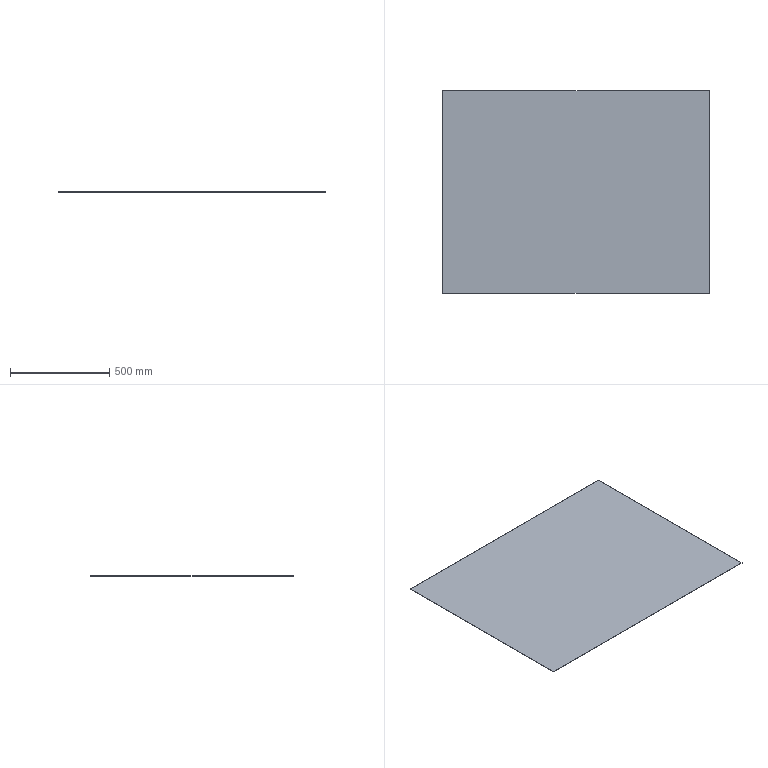Part | SolidWorks | features FlatPattern 1, SMBaseFlange 1, SheetMetal 1 | 1 solid | 6 faces | box 1345 x 1022 x 1.5 mm | volume 2062692 mm3 | plane 6
STEP:
#1=CARTESIAN_POINT('',(-672.5,0.,0.));
#2=VERTEX_POINT('',#1);
#3=CARTESIAN_POINT('',(-672.5,-1022.4,0.));
#4=VERTEX_POINT('',#3);
#5=CARTESIAN_POINT('',(-672.5,0.,0.));
#6=DIRECTION('',(0.,-1.,0.));
#7=VECTOR('',#6,1000.);
#8=LINE('',#5,#7);
#9=EDGE_CURVE('',#2,#4,#8,.T.);
#10=ORIENTED_EDGE('',*,*,#9,.T.);
#11=CARTESIAN_POINT('',(-672.5,-1022.4,1.5));
#12=VERTEX_POINT('',#11);
#13=CARTESIAN_POINT('',(-672.5,-1022.4,1.5));
#14=DIRECTION('',(0.,0.,-1.));
#15=VECTOR('',#14,1000.);
#16=LINE('',#13,#15);
#17=EDGE_CURVE('',#12,#4,#16,.T.);
#18=ORIENTED_EDGE('',*,*,#17,.F.);
#19=CARTESIAN_POINT('',(-672.5,0.,1.5));
#20=VERTEX_POINT('',#19);
#21=CARTESIAN_POINT('',(-672.5,0.,1.5));
#22=DIRECTION('',(0.,-1.,0.));
#23=VECTOR('',#22,1000.);
#24=LINE('',#21,#23);
#25=EDGE_CURVE('',#20,#12,#24,.T.);
#26=ORIENTED_EDGE('',*,*,#25,.F.);
#27=CARTESIAN_POINT('',(-672.5,0.,1.5));
#28=DIRECTION('',(0.,0.,-1.));
#29=VECTOR('',#28,1000.);
#30=LINE('',#27,#29);
#31=EDGE_CURVE('',#20,#2,#30,.T.);
#32=ORIENTED_EDGE('',*,*,#31,.T.);
#33=EDGE_LOOP('',(#10,#18,#26,#32));
#34=FACE_OUTER_BOUND('',#33,.T.);
#35=CARTESIAN_POINT('',(-672.5,0.,1.5));
#36=DIRECTION('',(1.,0.,0.));
#37=DIRECTION('',(0.,1.,0.));
#38=AXIS2_PLACEMENT_3D('',#35,#36,#37);
#39=PLANE('',#38);
#40=ADVANCED_FACE('',(#34),#39,.F.);
#41=CARTESIAN_POINT('',(672.5,-1022.4,0.));
#42=VERTEX_POINT('',#41);
#43=CARTESIAN_POINT('',(-672.5,-1022.4,0.));
#44=DIRECTION('',(1.,0.,0.));
#45=VECTOR('',#44,1000.);
#46=LINE('',#43,#45);
#47=EDGE_CURVE('',#4,#42,#46,.T.);
#48=ORIENTED_EDGE('',*,*,#47,.T.);
#49=CARTESIAN_POINT('',(672.5,-1022.4,1.5));
#50=VERTEX_POINT('',#49);
#51=CARTESIAN_POINT('',(672.5,-1022.4,1.5));
#52=DIRECTION('',(0.,0.,-1.));
#53=VECTOR('',#52,1000.);
#54=LINE('',#51,#53);
#55=EDGE_CURVE('',#50,#42,#54,.T.);
#56=ORIENTED_EDGE('',*,*,#55,.F.);
#57=CARTESIAN_POINT('',(-672.5,-1022.4,1.5));
#58=DIRECTION('',(1.,0.,0.));
#59=VECTOR('',#58,1000.);
#60=LINE('',#57,#59);
#61=EDGE_CURVE('',#12,#50,#60,.T.);
#62=ORIENTED_EDGE('',*,*,#61,.F.);
#63=ORIENTED_EDGE('',*,*,#17,.T.);
#64=EDGE_LOOP('',(#48,#56,#62,#63));
#65=FACE_OUTER_BOUND('',#64,.T.);
#66=CARTESIAN_POINT('',(-672.5,-1022.4,1.5));
#67=DIRECTION('',(0.,1.,0.));
#68=DIRECTION('',(0.,0.,1.));
#69=AXIS2_PLACEMENT_3D('',#66,#67,#68);
#70=PLANE('',#69);
#71=ADVANCED_FACE('',(#65),#70,.F.);
#72=CARTESIAN_POINT('',(672.5,0.,0.));
#73=VERTEX_POINT('',#72);
#74=CARTESIAN_POINT('',(672.5,0.,0.));
#75=DIRECTION('',(0.,1.,0.));
#76=VECTOR('',#75,1000.);
#77=LINE('',#74,#76);
#78=EDGE_CURVE('',#42,#73,#77,.T.);
#79=ORIENTED_EDGE('',*,*,#78,.T.);
#80=CARTESIAN_POINT('',(672.5,0.,1.5));
#81=VERTEX_POINT('',#80);
#82=CARTESIAN_POINT('',(672.5,0.,1.5));
#83=DIRECTION('',(0.,0.,-1.));
#84=VECTOR('',#83,1000.);
#85=LINE('',#82,#84);
#86=EDGE_CURVE('',#81,#73,#85,.T.);
#87=ORIENTED_EDGE('',*,*,#86,.F.);
#88=CARTESIAN_POINT('',(672.5,0.,1.5));
#89=DIRECTION('',(0.,1.,0.));
#90=VECTOR('',#89,1000.);
#91=LINE('',#88,#90);
#92=EDGE_CURVE('',#50,#81,#91,.T.);
#93=ORIENTED_EDGE('',*,*,#92,.F.);
#94=ORIENTED_EDGE('',*,*,#55,.T.);
#95=EDGE_LOOP('',(#79,#87,#93,#94));
#96=FACE_OUTER_BOUND('',#95,.T.);
#97=CARTESIAN_POINT('',(672.5,0.,1.5));
#98=DIRECTION('',(-1.,0.,0.));
#99=DIRECTION('',(0.,-1.,0.));
#100=AXIS2_PLACEMENT_3D('',#97,#98,#99);
#101=PLANE('',#100);
#102=ADVANCED_FACE('',(#96),#101,.F.);
#103=CARTESIAN_POINT('',(-672.5,0.,0.));
#104=DIRECTION('',(-1.,0.,0.));
#105=VECTOR('',#104,1000.);
#106=LINE('',#103,#105);
#107=EDGE_CURVE('',#73,#2,#106,.T.);
#108=ORIENTED_EDGE('',*,*,#107,.T.);
#109=ORIENTED_EDGE('',*,*,#31,.F.);
#110=CARTESIAN_POINT('',(-672.5,0.,1.5));
#111=DIRECTION('',(-1.,0.,0.));
#112=VECTOR('',#111,1000.);
#113=LINE('',#110,#112);
#114=EDGE_CURVE('',#81,#20,#113,.T.);
#115=ORIENTED_EDGE('',*,*,#114,.F.);
#116=ORIENTED_EDGE('',*,*,#86,.T.);
#117=EDGE_LOOP('',(#108,#109,#115,#116));
#118=FACE_OUTER_BOUND('',#117,.T.);
#119=CARTESIAN_POINT('',(-672.5,0.,1.5));
#120=DIRECTION('',(0.,-1.,0.));
#121=DIRECTION('',(1.,0.,0.));
#122=AXIS2_PLACEMENT_3D('',#119,#120,#121);
#123=PLANE('',#122);
#124=ADVANCED_FACE('',(#118),#123,.F.);
#125=ORIENTED_EDGE('',*,*,#25,.T.);
#126=ORIENTED_EDGE('',*,*,#61,.T.);
#127=ORIENTED_EDGE('',*,*,#92,.T.);
#128=ORIENTED_EDGE('',*,*,#114,.T.);
#129=EDGE_LOOP('',(#125,#126,#127,#128));
#130=FACE_OUTER_BOUND('',#129,.T.);
#131=CARTESIAN_POINT('',(0.,0.,1.5));
#132=DIRECTION('',(0.,0.,1.));
#133=DIRECTION('',(1.,0.,0.));
#134=AXIS2_PLACEMENT_3D('',#131,#132,#133);
#135=PLANE('',#134);
#136=ADVANCED_FACE('',(#130),#135,.T.);
#137=ORIENTED_EDGE('',*,*,#9,.F.);
#138=ORIENTED_EDGE('',*,*,#107,.F.);
#139=ORIENTED_EDGE('',*,*,#78,.F.);
#140=ORIENTED_EDGE('',*,*,#47,.F.);
#141=EDGE_LOOP('',(#137,#138,#139,#140));
#142=FACE_OUTER_BOUND('',#141,.T.);
#143=CARTESIAN_POINT('',(0.,0.,0.));
#144=DIRECTION('',(0.,0.,1.));
#145=DIRECTION('',(1.,0.,0.));
#146=AXIS2_PLACEMENT_3D('',#143,#144,#145);
#147=PLANE('',#146);
#148=ADVANCED_FACE('',(#142),#147,.F.);
#149=CLOSED_SHELL('',(#40,#71,#102,#124,#136,#148));
#150=MANIFOLD_SOLID_BREP('',#149);
#151=CARTESIAN_POINT('',(0.,0.,0.));
#152=DIRECTION('',(0.,0.,1.));
#153=DIRECTION('',(1.,0.,0.));
#154=AXIS2_PLACEMENT_3D('',#151,#152,#153);
#155=(LENGTH_UNIT()NAMED_UNIT(*)SI_UNIT(.MILLI.,.METRE.));
#156=UNCERTAINTY_MEASURE_WITH_UNIT(LENGTH_MEASURE(0.00001),#155,'','');
#157=(NAMED_UNIT(*)PLANE_ANGLE_UNIT()SI_UNIT($,.RADIAN.));
#158=(NAMED_UNIT(*)SI_UNIT($,.STERADIAN.)SOLID_ANGLE_UNIT());
#159=(GEOMETRIC_REPRESENTATION_CONTEXT(3)GLOBAL_UNCERTAINTY_ASSIGNED_CONTEXT((#156))GLOBAL_UNIT_ASSIGNED_CONTEXT((#155,#157,#158))REPRESENTATION_CONTEXT('',''));
#160=ADVANCED_BREP_SHAPE_REPRESENTATION('',(#150,#154),#159);